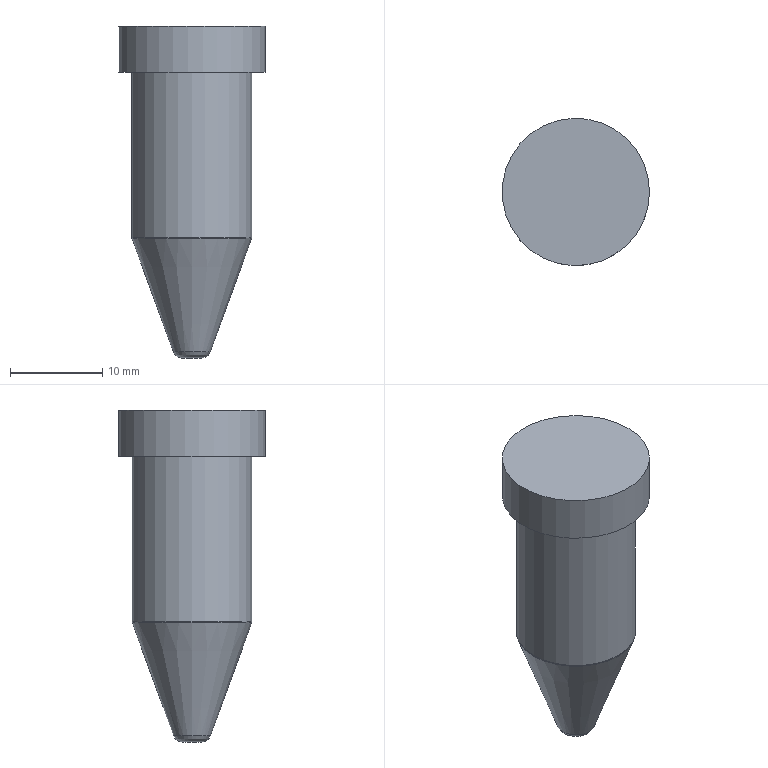Part | NX | features solid 2 | 1 solid | 8 faces | box 16 x 16 x 36.053 mm | volume 4175 mm3 | plane 3 | cylinder 2 | torus 2 | cone 1 | commonest cylinder face diameters 13 x1 16 x1
STEP:
#1=CARTESIAN_POINT('',(684.068,0.,-16.053));
#2=VERTEX_POINT('',#1);
#3=CARTESIAN_POINT('',(683.,0.,-16.053));
#4=DIRECTION('',(0.,0.,1.));
#5=DIRECTION('',(1.,0.,0.));
#6=AXIS2_PLACEMENT_3D('',#3,#4,#5);
#7=CIRCLE('',#6,1.068);
#8=EDGE_CURVE('',#2,#2,#7,.F.);
#9=ORIENTED_EDGE('',*,*,#8,.T.);
#10=EDGE_LOOP('',(#9));
#11=FACE_BOUND('',#10,.T.);
#12=CARTESIAN_POINT('',(683.,0.,-16.053));
#13=DIRECTION('',(0.,0.,-1.));
#14=DIRECTION('',(1.,0.,0.));
#15=AXIS2_PLACEMENT_3D('',#12,#13,#14);
#16=PLANE('',#15);
#17=ADVANCED_FACE('',(#11),#16,.T.);
#18=CARTESIAN_POINT('',(691.,0.,20.));
#19=VERTEX_POINT('',#18);
#20=CARTESIAN_POINT('',(683.,0.,20.));
#21=DIRECTION('',(0.,0.,1.));
#22=DIRECTION('',(1.,0.,0.));
#23=AXIS2_PLACEMENT_3D('',#20,#21,#22);
#24=CIRCLE('',#23,8.);
#25=EDGE_CURVE('',#19,#19,#24,.F.);
#26=ORIENTED_EDGE('',*,*,#25,.F.);
#27=EDGE_LOOP('',(#26));
#28=FACE_BOUND('',#27,.T.);
#29=CARTESIAN_POINT('',(704.285,-110.548,20.));
#30=DIRECTION('',(0.,0.,1.));
#31=DIRECTION('',(1.,0.,0.));
#32=AXIS2_PLACEMENT_3D('',#29,#30,#31);
#33=PLANE('',#32);
#34=ADVANCED_FACE('',(#28),#33,.T.);
#35=CARTESIAN_POINT('',(689.5,0.,-3.));
#36=VERTEX_POINT('',#35);
#37=CARTESIAN_POINT('',(683.,0.,-3.));
#38=DIRECTION('',(0.,0.,1.));
#39=DIRECTION('',(1.,0.,0.));
#40=AXIS2_PLACEMENT_3D('',#37,#38,#39);
#41=CIRCLE('',#40,6.5);
#42=EDGE_CURVE('',#36,#36,#41,.T.);
#43=ORIENTED_EDGE('',*,*,#42,.T.);
#44=EDGE_LOOP('',(#43));
#45=FACE_BOUND('',#44,.T.);
#46=CARTESIAN_POINT('',(689.5,0.,15.));
#47=VERTEX_POINT('',#46);
#48=CARTESIAN_POINT('',(683.,0.,15.));
#49=DIRECTION('',(0.,0.,1.));
#50=DIRECTION('',(1.,0.,0.));
#51=AXIS2_PLACEMENT_3D('',#48,#49,#50);
#52=CIRCLE('',#51,6.5);
#53=EDGE_CURVE('',#47,#47,#52,.F.);
#54=ORIENTED_EDGE('',*,*,#53,.T.);
#55=EDGE_LOOP('',(#54));
#56=FACE_BOUND('',#55,.T.);
#57=CARTESIAN_POINT('',(683.,0.,13.947));
#58=DIRECTION('',(0.,0.,-1.));
#59=DIRECTION('',(1.,0.,0.));
#60=AXIS2_PLACEMENT_3D('',#57,#58,#59);
#61=CYLINDRICAL_SURFACE('',#60,6.5);
#62=ADVANCED_FACE('',(#45,#56),#61,.T.);
#63=ORIENTED_EDGE('',*,*,#53,.F.);
#64=EDGE_LOOP('',(#63));
#65=FACE_BOUND('',#64,.T.);
#66=CARTESIAN_POINT('',(691.,0.,15.));
#67=VERTEX_POINT('',#66);
#68=CARTESIAN_POINT('',(683.,0.,15.));
#69=DIRECTION('',(0.,0.,1.));
#70=DIRECTION('',(1.,0.,0.));
#71=AXIS2_PLACEMENT_3D('',#68,#69,#70);
#72=CIRCLE('',#71,8.);
#73=EDGE_CURVE('',#67,#67,#72,.T.);
#74=ORIENTED_EDGE('',*,*,#73,.F.);
#75=EDGE_LOOP('',(#74));
#76=FACE_BOUND('',#75,.T.);
#77=CARTESIAN_POINT('',(683.,0.,15.));
#78=DIRECTION('',(0.,0.,-1.));
#79=DIRECTION('',(1.,0.,0.));
#80=AXIS2_PLACEMENT_3D('',#77,#78,#79);
#81=PLANE('',#80);
#82=ADVANCED_FACE('',(#65,#76),#81,.T.);
#83=ORIENTED_EDGE('',*,*,#73,.T.);
#84=EDGE_LOOP('',(#83));
#85=FACE_BOUND('',#84,.T.);
#86=ORIENTED_EDGE('',*,*,#25,.T.);
#87=EDGE_LOOP('',(#86));
#88=FACE_BOUND('',#87,.T.);
#89=CARTESIAN_POINT('',(683.,0.,16.947));
#90=DIRECTION('',(0.,0.,-1.));
#91=DIRECTION('',(1.,0.,0.));
#92=AXIS2_PLACEMENT_3D('',#89,#90,#91);
#93=CYLINDRICAL_SURFACE('',#92,8.);
#94=ADVANCED_FACE('',(#85,#88),#93,.T.);
#95=CARTESIAN_POINT('',(689.482,0.,-3.103));
#96=VERTEX_POINT('',#95);
#97=CARTESIAN_POINT('',(683.,0.,-3.103));
#98=DIRECTION('',(0.,0.,1.));
#99=DIRECTION('',(1.,0.,0.));
#100=AXIS2_PLACEMENT_3D('',#97,#98,#99);
#101=CIRCLE('',#100,6.482);
#102=EDGE_CURVE('',#96,#96,#101,.F.);
#103=ORIENTED_EDGE('',*,*,#102,.T.);
#104=EDGE_LOOP('',(#103));
#105=FACE_BOUND('',#104,.T.);
#106=CARTESIAN_POINT('',(685.008,0.,-15.395));
#107=VERTEX_POINT('',#106);
#108=CARTESIAN_POINT('',(683.,0.,-15.395));
#109=DIRECTION('',(0.,0.,1.));
#110=DIRECTION('',(1.,0.,0.));
#111=AXIS2_PLACEMENT_3D('',#108,#109,#110);
#112=CIRCLE('',#111,2.008);
#113=EDGE_CURVE('',#107,#107,#112,.T.);
#114=ORIENTED_EDGE('',*,*,#113,.T.);
#115=EDGE_LOOP('',(#114));
#116=FACE_BOUND('',#115,.T.);
#117=CARTESIAN_POINT('',(683.,0.,-16.053));
#118=DIRECTION('',(0.,0.,1.));
#119=DIRECTION('',(-1.,0.,0.));
#120=AXIS2_PLACEMENT_3D('',#117,#118,#119);
#121=CONICAL_SURFACE('',#120,1.768,0.3491);
#122=ADVANCED_FACE('',(#105,#116),#121,.T.);
#123=ORIENTED_EDGE('',*,*,#113,.F.);
#124=EDGE_LOOP('',(#123));
#125=FACE_BOUND('',#124,.T.);
#126=ORIENTED_EDGE('',*,*,#8,.F.);
#127=EDGE_LOOP('',(#126));
#128=FACE_BOUND('',#127,.T.);
#129=CARTESIAN_POINT('',(683.,0.,-15.053));
#130=DIRECTION('',(0.,0.,-1.));
#131=DIRECTION('',(1.,0.,0.));
#132=AXIS2_PLACEMENT_3D('',#129,#130,#131);
#133=TOROIDAL_SURFACE('',#132,1.068,1.);
#134=ADVANCED_FACE('',(#125,#128),#133,.T.);
#135=ORIENTED_EDGE('',*,*,#102,.F.);
#136=EDGE_LOOP('',(#135));
#137=FACE_BOUND('',#136,.T.);
#138=ORIENTED_EDGE('',*,*,#42,.F.);
#139=EDGE_LOOP('',(#138));
#140=FACE_BOUND('',#139,.T.);
#141=CARTESIAN_POINT('',(683.,0.,-3.));
#142=DIRECTION('',(0.,0.,-1.));
#143=DIRECTION('',(1.,0.,0.));
#144=AXIS2_PLACEMENT_3D('',#141,#142,#143);
#145=TOROIDAL_SURFACE('',#144,6.2,0.3);
#146=ADVANCED_FACE('',(#137,#140),#145,.T.);
#147=CLOSED_SHELL('',(#17,#34,#62,#82,#94,#122,#134,#146));
#148=MANIFOLD_SOLID_BREP('',#147);
#149=(LENGTH_UNIT()NAMED_UNIT(*)SI_UNIT(.MILLI.,.METRE.));
#150=UNCERTAINTY_MEASURE_WITH_UNIT(LENGTH_MEASURE(0.00001),#149,'','');
#151=(NAMED_UNIT(*)PLANE_ANGLE_UNIT()SI_UNIT($,.RADIAN.));
#152=(NAMED_UNIT(*)SI_UNIT($,.STERADIAN.)SOLID_ANGLE_UNIT());
#153=(GEOMETRIC_REPRESENTATION_CONTEXT(3)GLOBAL_UNCERTAINTY_ASSIGNED_CONTEXT((#150))GLOBAL_UNIT_ASSIGNED_CONTEXT((#149,#151,#152))REPRESENTATION_CONTEXT('',''));
#154=ADVANCED_BREP_SHAPE_REPRESENTATION('',(#148),#153);